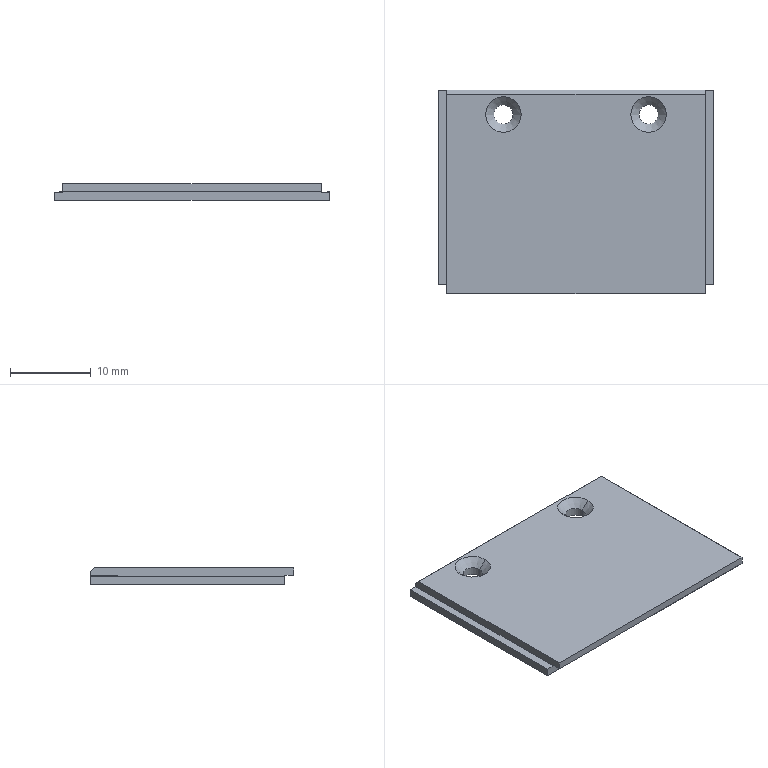Part | STEP file | ASND-0110-OPT-CO40-X-V1.0 lower cover plate | 1 solid | 21 faces | box 34 x 25.2 x 2 mm | volume 1591 mm3 | plane 13 | cone 4 | cylinder 4 | commonest cylinder face diameters 2.4 x4